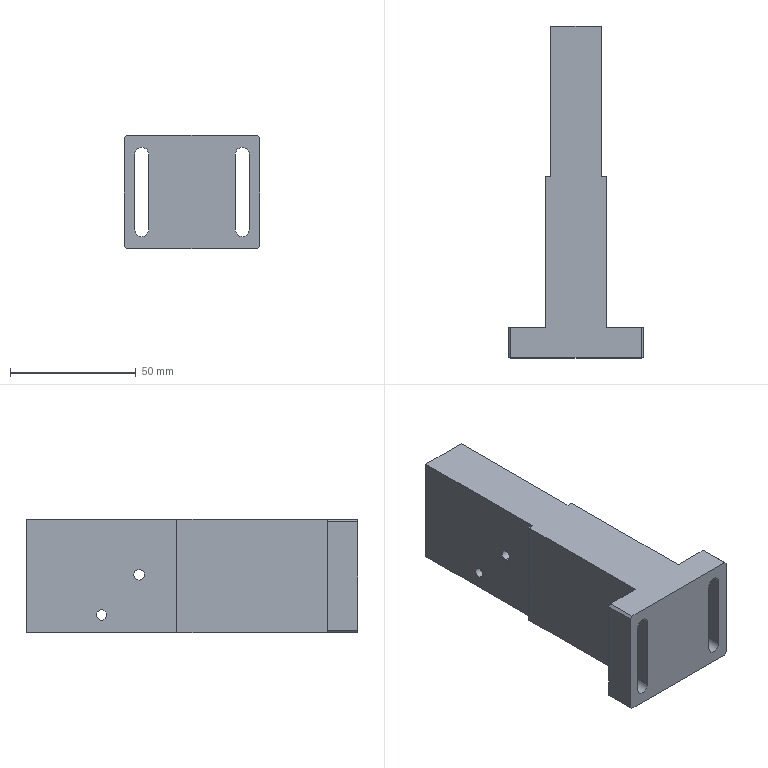Part | SolidWorks | features HoleWzd 3, ICE 2, Chamfer 1, Extrusion 1 | 1 solid | 40 faces | box 54 x 132 x 45 mm | volume 142452 mm3 | plane 22 | cylinder 14 | cone 4 | commonest cylinder face diameters 4.2 x8 5.5 x6
STEP:
#1=CARTESIAN_POINT('',(0.,118.,35.4));
#2=VERTEX_POINT('',#1);
#3=CARTESIAN_POINT('',(0.,118.,39.6));
#4=VERTEX_POINT('',#3);
#5=CARTESIAN_POINT('',(0.,118.,37.5));
#6=DIRECTION('',(0.,1.,0.));
#7=DIRECTION('',(0.,0.,1.));
#8=AXIS2_PLACEMENT_3D('',#5,#6,#7);
#9=CIRCLE('',#8,2.1);
#10=EDGE_CURVE('',#2,#4,#9,.T.);
#11=ORIENTED_EDGE('',*,*,#10,.F.);
#12=CARTESIAN_POINT('',(0.,132.,35.4));
#13=VERTEX_POINT('',#12);
#14=CARTESIAN_POINT('',(0.,132.,35.4));
#15=DIRECTION('',(0.,1.,0.));
#16=VECTOR('',#15,1000.);
#17=LINE('',#14,#16);
#18=EDGE_CURVE('',#2,#13,#17,.T.);
#19=ORIENTED_EDGE('',*,*,#18,.T.);
#20=CARTESIAN_POINT('',(0.,132.,39.6));
#21=VERTEX_POINT('',#20);
#22=CARTESIAN_POINT('',(0.,132.,37.5));
#23=DIRECTION('',(0.,1.,0.));
#24=DIRECTION('',(0.,0.,1.));
#25=AXIS2_PLACEMENT_3D('',#22,#23,#24);
#26=CIRCLE('',#25,2.1);
#27=EDGE_CURVE('',#13,#21,#26,.T.);
#28=ORIENTED_EDGE('',*,*,#27,.T.);
#29=CARTESIAN_POINT('',(0.,132.,39.6));
#30=DIRECTION('',(0.,1.,0.));
#31=VECTOR('',#30,1000.);
#32=LINE('',#29,#31);
#33=EDGE_CURVE('',#4,#21,#32,.T.);
#34=ORIENTED_EDGE('',*,*,#33,.F.);
#35=EDGE_LOOP('',(#11,#19,#28,#34));
#36=FACE_OUTER_BOUND('',#35,.T.);
#37=CARTESIAN_POINT('',(0.,132.,37.5));
#38=DIRECTION('',(0.,1.,0.));
#39=DIRECTION('',(0.,0.,1.));
#40=AXIS2_PLACEMENT_3D('',#37,#38,#39);
#41=CYLINDRICAL_SURFACE('',#40,2.1);
#42=ADVANCED_FACE('',(#36),#41,.F.);
#43=CARTESIAN_POINT('',(0.,116.738,37.5));
#44=VERTEX_POINT('',#43);
#45=CARTESIAN_POINT('',(0.,118.,39.6));
#46=DIRECTION('',(0.,0.515,0.8572));
#47=VECTOR('',#46,1000.);
#48=LINE('',#45,#47);
#49=EDGE_CURVE('',#44,#4,#48,.T.);
#50=ORIENTED_EDGE('',*,*,#49,.F.);
#51=CARTESIAN_POINT('',(0.,118.,35.4));
#52=DIRECTION('',(0.,0.515,-0.8572));
#53=VECTOR('',#52,1000.);
#54=LINE('',#51,#53);
#55=EDGE_CURVE('',#44,#2,#54,.T.);
#56=ORIENTED_EDGE('',*,*,#55,.T.);
#57=ORIENTED_EDGE('',*,*,#10,.T.);
#58=EDGE_LOOP('',(#50,#56,#57));
#59=FACE_OUTER_BOUND('',#58,.T.);
#60=CARTESIAN_POINT('',(0.,118.,37.5));
#61=DIRECTION('',(0.,1.,0.));
#62=DIRECTION('',(0.,0.,1.));
#63=AXIS2_PLACEMENT_3D('',#60,#61,#62);
#64=CONICAL_SURFACE('',#63,2.1,1.03);
#65=ADVANCED_FACE('',(#59),#64,.F.);
#66=CARTESIAN_POINT('',(0.,118.,5.4));
#67=VERTEX_POINT('',#66);
#68=CARTESIAN_POINT('',(0.,118.,9.6));
#69=VERTEX_POINT('',#68);
#70=CARTESIAN_POINT('',(0.,118.,7.5));
#71=DIRECTION('',(0.,1.,0.));
#72=DIRECTION('',(0.,0.,1.));
#73=AXIS2_PLACEMENT_3D('',#70,#71,#72);
#74=CIRCLE('',#73,2.1);
#75=EDGE_CURVE('',#67,#69,#74,.T.);
#76=ORIENTED_EDGE('',*,*,#75,.F.);
#77=CARTESIAN_POINT('',(0.,132.,5.4));
#78=VERTEX_POINT('',#77);
#79=CARTESIAN_POINT('',(0.,132.,5.4));
#80=DIRECTION('',(0.,1.,0.));
#81=VECTOR('',#80,1000.);
#82=LINE('',#79,#81);
#83=EDGE_CURVE('',#67,#78,#82,.T.);
#84=ORIENTED_EDGE('',*,*,#83,.T.);
#85=CARTESIAN_POINT('',(0.,132.,9.6));
#86=VERTEX_POINT('',#85);
#87=CARTESIAN_POINT('',(0.,132.,7.5));
#88=DIRECTION('',(0.,1.,0.));
#89=DIRECTION('',(0.,0.,1.));
#90=AXIS2_PLACEMENT_3D('',#87,#88,#89);
#91=CIRCLE('',#90,2.1);
#92=EDGE_CURVE('',#78,#86,#91,.T.);
#93=ORIENTED_EDGE('',*,*,#92,.T.);
#94=CARTESIAN_POINT('',(0.,132.,9.6));
#95=DIRECTION('',(0.,1.,0.));
#96=VECTOR('',#95,1000.);
#97=LINE('',#94,#96);
#98=EDGE_CURVE('',#69,#86,#97,.T.);
#99=ORIENTED_EDGE('',*,*,#98,.F.);
#100=EDGE_LOOP('',(#76,#84,#93,#99));
#101=FACE_OUTER_BOUND('',#100,.T.);
#102=CARTESIAN_POINT('',(0.,132.,7.5));
#103=DIRECTION('',(0.,1.,0.));
#104=DIRECTION('',(0.,0.,1.));
#105=AXIS2_PLACEMENT_3D('',#102,#103,#104);
#106=CYLINDRICAL_SURFACE('',#105,2.1);
#107=ADVANCED_FACE('',(#101),#106,.F.);
#108=CARTESIAN_POINT('',(0.,116.738,7.5));
#109=VERTEX_POINT('',#108);
#110=CARTESIAN_POINT('',(0.,118.,9.6));
#111=DIRECTION('',(0.,0.515,0.8572));
#112=VECTOR('',#111,1000.);
#113=LINE('',#110,#112);
#114=EDGE_CURVE('',#109,#69,#113,.T.);
#115=ORIENTED_EDGE('',*,*,#114,.F.);
#116=CARTESIAN_POINT('',(0.,118.,5.4));
#117=DIRECTION('',(0.,0.515,-0.8572));
#118=VECTOR('',#117,1000.);
#119=LINE('',#116,#118);
#120=EDGE_CURVE('',#109,#67,#119,.T.);
#121=ORIENTED_EDGE('',*,*,#120,.T.);
#122=ORIENTED_EDGE('',*,*,#75,.T.);
#123=EDGE_LOOP('',(#115,#121,#122));
#124=FACE_OUTER_BOUND('',#123,.T.);
#125=CARTESIAN_POINT('',(0.,118.,7.5));
#126=DIRECTION('',(0.,1.,0.));
#127=DIRECTION('',(0.,0.,1.));
#128=AXIS2_PLACEMENT_3D('',#125,#126,#127);
#129=CONICAL_SURFACE('',#128,2.1,1.03);
#130=ADVANCED_FACE('',(#124),#129,.F.);
#131=CARTESIAN_POINT('',(-20.,0.,40.25));
#132=VERTEX_POINT('',#131);
#133=CARTESIAN_POINT('',(-17.25,0.,37.5));
#134=VERTEX_POINT('',#133);
#135=CARTESIAN_POINT('',(-20.,0.,37.5));
#136=DIRECTION('',(0.,1.,0.));
#137=DIRECTION('',(0.,0.,1.));
#138=AXIS2_PLACEMENT_3D('',#135,#136,#137);
#139=CIRCLE('',#138,2.75);
#140=EDGE_CURVE('',#132,#134,#139,.T.);
#141=ORIENTED_EDGE('',*,*,#140,.F.);
#142=CARTESIAN_POINT('',(-20.,12.,40.25));
#143=VERTEX_POINT('',#142);
#144=CARTESIAN_POINT('',(-20.,12.,40.25));
#145=DIRECTION('',(0.,1.,0.));
#146=VECTOR('',#145,1000.);
#147=LINE('',#144,#146);
#148=EDGE_CURVE('',#132,#143,#147,.T.);
#149=ORIENTED_EDGE('',*,*,#148,.T.);
#150=CARTESIAN_POINT('',(-17.25,12.,37.5));
#151=VERTEX_POINT('',#150);
#152=CARTESIAN_POINT('',(-20.,12.,37.5));
#153=DIRECTION('',(0.,1.,0.));
#154=DIRECTION('',(0.,0.,1.));
#155=AXIS2_PLACEMENT_3D('',#152,#153,#154);
#156=CIRCLE('',#155,2.75);
#157=EDGE_CURVE('',#143,#151,#156,.T.);
#158=ORIENTED_EDGE('',*,*,#157,.T.);
#159=CARTESIAN_POINT('',(-17.25,12.,37.5));
#160=DIRECTION('',(0.,1.,0.));
#161=VECTOR('',#160,1000.);
#162=LINE('',#159,#161);
#163=EDGE_CURVE('',#134,#151,#162,.T.);
#164=ORIENTED_EDGE('',*,*,#163,.F.);
#165=EDGE_LOOP('',(#141,#149,#158,#164));
#166=FACE_OUTER_BOUND('',#165,.T.);
#167=CARTESIAN_POINT('',(-20.,12.,37.5));
#168=DIRECTION('',(0.,1.,0.));
#169=DIRECTION('',(0.,0.,1.));
#170=AXIS2_PLACEMENT_3D('',#167,#168,#169);
#171=CYLINDRICAL_SURFACE('',#170,2.75);
#172=ADVANCED_FACE('',(#166),#171,.F.);
#173=CARTESIAN_POINT('',(20.,0.,40.25));
#174=VERTEX_POINT('',#173);
#175=CARTESIAN_POINT('',(22.75,0.,37.5));
#176=VERTEX_POINT('',#175);
#177=CARTESIAN_POINT('',(20.,0.,37.5));
#178=DIRECTION('',(0.,1.,0.));
#179=DIRECTION('',(0.,0.,1.));
#180=AXIS2_PLACEMENT_3D('',#177,#178,#179);
#181=CIRCLE('',#180,2.75);
#182=EDGE_CURVE('',#174,#176,#181,.T.);
#183=ORIENTED_EDGE('',*,*,#182,.F.);
#184=CARTESIAN_POINT('',(20.,12.,40.25));
#185=VERTEX_POINT('',#184);
#186=CARTESIAN_POINT('',(20.,12.,40.25));
#187=DIRECTION('',(0.,1.,0.));
#188=VECTOR('',#187,1000.);
#189=LINE('',#186,#188);
#190=EDGE_CURVE('',#174,#185,#189,.T.);
#191=ORIENTED_EDGE('',*,*,#190,.T.);
#192=CARTESIAN_POINT('',(22.75,12.,37.5));
#193=VERTEX_POINT('',#192);
#194=CARTESIAN_POINT('',(20.,12.,37.5));
#195=DIRECTION('',(0.,1.,0.));
#196=DIRECTION('',(0.,0.,1.));
#197=AXIS2_PLACEMENT_3D('',#194,#195,#196);
#198=CIRCLE('',#197,2.75);
#199=EDGE_CURVE('',#185,#193,#198,.T.);
#200=ORIENTED_EDGE('',*,*,#199,.T.);
#201=CARTESIAN_POINT('',(22.75,12.,37.5));
#202=DIRECTION('',(0.,1.,0.));
#203=VECTOR('',#202,1000.);
#204=LINE('',#201,#203);
#205=EDGE_CURVE('',#176,#193,#204,.T.);
#206=ORIENTED_EDGE('',*,*,#205,.F.);
#207=EDGE_LOOP('',(#183,#191,#200,#206));
#208=FACE_OUTER_BOUND('',#207,.T.);
#209=CARTESIAN_POINT('',(20.,12.,37.5));
#210=DIRECTION('',(0.,1.,0.));
#211=DIRECTION('',(0.,0.,1.));
#212=AXIS2_PLACEMENT_3D('',#209,#210,#211);
#213=CYLINDRICAL_SURFACE('',#212,2.75);
#214=ADVANCED_FACE('',(#208),#213,.F.);
#215=CARTESIAN_POINT('',(-10.,102.,9.1));
#216=VERTEX_POINT('',#215);
#217=CARTESIAN_POINT('',(-10.,102.,4.9));
#218=VERTEX_POINT('',#217);
#219=CARTESIAN_POINT('',(-10.,102.,7.));
#220=DIRECTION('',(1.,0.,0.));
#221=DIRECTION('',(0.,1.,0.));
#222=AXIS2_PLACEMENT_3D('',#219,#220,#221);
#223=CIRCLE('',#222,2.1);
#224=EDGE_CURVE('',#216,#218,#223,.T.);
#225=ORIENTED_EDGE('',*,*,#224,.F.);
#226=CARTESIAN_POINT('',(10.,102.,9.1));
#227=VERTEX_POINT('',#226);
#228=CARTESIAN_POINT('',(10.,102.,9.1));
#229=DIRECTION('',(1.,0.,0.));
#230=VECTOR('',#229,1000.);
#231=LINE('',#228,#230);
#232=EDGE_CURVE('',#216,#227,#231,.T.);
#233=ORIENTED_EDGE('',*,*,#232,.T.);
#234=CARTESIAN_POINT('',(10.,102.,4.9));
#235=VERTEX_POINT('',#234);
#236=CARTESIAN_POINT('',(10.,102.,7.));
#237=DIRECTION('',(1.,0.,0.));
#238=DIRECTION('',(0.,0.,-1.));
#239=AXIS2_PLACEMENT_3D('',#236,#237,#238);
#240=CIRCLE('',#239,2.1);
#241=EDGE_CURVE('',#227,#235,#240,.T.);
#242=ORIENTED_EDGE('',*,*,#241,.T.);
#243=CARTESIAN_POINT('',(10.,102.,4.9));
#244=DIRECTION('',(1.,0.,0.));
#245=VECTOR('',#244,1000.);
#246=LINE('',#243,#245);
#247=EDGE_CURVE('',#218,#235,#246,.T.);
#248=ORIENTED_EDGE('',*,*,#247,.F.);
#249=EDGE_LOOP('',(#225,#233,#242,#248));
#250=FACE_OUTER_BOUND('',#249,.T.);
#251=CARTESIAN_POINT('',(10.,102.,7.));
#252=DIRECTION('',(1.,0.,0.));
#253=DIRECTION('',(0.,0.,-1.));
#254=AXIS2_PLACEMENT_3D('',#251,#252,#253);
#255=CYLINDRICAL_SURFACE('',#254,2.1);
#256=ADVANCED_FACE('',(#250),#255,.F.);
#257=CARTESIAN_POINT('',(-10.,87.,25.1));
#258=VERTEX_POINT('',#257);
#259=CARTESIAN_POINT('',(-10.,87.,20.9));
#260=VERTEX_POINT('',#259);
#261=CARTESIAN_POINT('',(-10.,87.,23.));
#262=DIRECTION('',(1.,0.,0.));
#263=DIRECTION('',(0.,1.,0.));
#264=AXIS2_PLACEMENT_3D('',#261,#262,#263);
#265=CIRCLE('',#264,2.1);
#266=EDGE_CURVE('',#258,#260,#265,.T.);
#267=ORIENTED_EDGE('',*,*,#266,.F.);
#268=CARTESIAN_POINT('',(10.,87.,25.1));
#269=VERTEX_POINT('',#268);
#270=CARTESIAN_POINT('',(10.,87.,25.1));
#271=DIRECTION('',(1.,0.,0.));
#272=VECTOR('',#271,1000.);
#273=LINE('',#270,#272);
#274=EDGE_CURVE('',#258,#269,#273,.T.);
#275=ORIENTED_EDGE('',*,*,#274,.T.);
#276=CARTESIAN_POINT('',(10.,87.,20.9));
#277=VERTEX_POINT('',#276);
#278=CARTESIAN_POINT('',(10.,87.,23.));
#279=DIRECTION('',(1.,0.,0.));
#280=DIRECTION('',(0.,0.,-1.));
#281=AXIS2_PLACEMENT_3D('',#278,#279,#280);
#282=CIRCLE('',#281,2.1);
#283=EDGE_CURVE('',#269,#277,#282,.T.);
#284=ORIENTED_EDGE('',*,*,#283,.T.);
#285=CARTESIAN_POINT('',(10.,87.,20.9));
#286=DIRECTION('',(1.,0.,0.));
#287=VECTOR('',#286,1000.);
#288=LINE('',#285,#287);
#289=EDGE_CURVE('',#260,#277,#288,.T.);
#290=ORIENTED_EDGE('',*,*,#289,.F.);
#291=EDGE_LOOP('',(#267,#275,#284,#290));
#292=FACE_OUTER_BOUND('',#291,.T.);
#293=CARTESIAN_POINT('',(10.,87.,23.));
#294=DIRECTION('',(1.,0.,0.));
#295=DIRECTION('',(0.,0.,-1.));
#296=AXIS2_PLACEMENT_3D('',#293,#294,#295);
#297=CYLINDRICAL_SURFACE('',#296,2.1);
#298=ADVANCED_FACE('',(#292),#297,.F.);
#299=CARTESIAN_POINT('',(22.75,0.,7.5));
#300=VERTEX_POINT('',#299);
#301=CARTESIAN_POINT('',(22.75,12.,7.5));
#302=VERTEX_POINT('',#301);
#303=CARTESIAN_POINT('',(22.75,12.,7.5));
#304=DIRECTION('',(0.,1.,0.));
#305=VECTOR('',#304,1000.);
#306=LINE('',#303,#305);
#307=EDGE_CURVE('',#300,#302,#306,.T.);
#308=ORIENTED_EDGE('',*,*,#307,.T.);
#309=CARTESIAN_POINT('',(17.25,12.,7.5));
#310=VERTEX_POINT('',#309);
#311=CARTESIAN_POINT('',(20.,12.,7.5));
#312=DIRECTION('',(0.,1.,0.));
#313=DIRECTION('',(0.,0.,1.));
#314=AXIS2_PLACEMENT_3D('',#311,#312,#313);
#315=CIRCLE('',#314,2.75);
#316=EDGE_CURVE('',#302,#310,#315,.T.);
#317=ORIENTED_EDGE('',*,*,#316,.T.);
#318=CARTESIAN_POINT('',(17.25,0.,7.5));
#319=VERTEX_POINT('',#318);
#320=CARTESIAN_POINT('',(17.25,12.,7.5));
#321=DIRECTION('',(0.,1.,0.));
#322=VECTOR('',#321,1000.);
#323=LINE('',#320,#322);
#324=EDGE_CURVE('',#319,#310,#323,.T.);
#325=ORIENTED_EDGE('',*,*,#324,.F.);
#326=CARTESIAN_POINT('',(20.,0.,7.5));
#327=DIRECTION('',(0.,1.,0.));
#328=DIRECTION('',(0.,0.,1.));
#329=AXIS2_PLACEMENT_3D('',#326,#327,#328);
#330=CIRCLE('',#329,2.75);
#331=EDGE_CURVE('',#300,#319,#330,.T.);
#332=ORIENTED_EDGE('',*,*,#331,.F.);
#333=EDGE_LOOP('',(#308,#317,#325,#332));
#334=FACE_OUTER_BOUND('',#333,.T.);
#335=CARTESIAN_POINT('',(20.,12.,7.5));
#336=DIRECTION('',(0.,1.,0.));
#337=DIRECTION('',(0.,0.,1.));
#338=AXIS2_PLACEMENT_3D('',#335,#336,#337);
#339=CYLINDRICAL_SURFACE('',#338,2.75);
#340=ADVANCED_FACE('',(#334),#339,.F.);
#341=CARTESIAN_POINT('',(-17.25,0.,7.5));
#342=VERTEX_POINT('',#341);
#343=CARTESIAN_POINT('',(-17.25,12.,7.5));
#344=VERTEX_POINT('',#343);
#345=CARTESIAN_POINT('',(-17.25,12.,7.5));
#346=DIRECTION('',(0.,1.,0.));
#347=VECTOR('',#346,1000.);
#348=LINE('',#345,#347);
#349=EDGE_CURVE('',#342,#344,#348,.T.);
#350=ORIENTED_EDGE('',*,*,#349,.T.);
#351=CARTESIAN_POINT('',(-22.75,12.,7.5));
#352=VERTEX_POINT('',#351);
#353=CARTESIAN_POINT('',(-20.,12.,7.5));
#354=DIRECTION('',(0.,1.,0.));
#355=DIRECTION('',(0.,0.,1.));
#356=AXIS2_PLACEMENT_3D('',#353,#354,#355);
#357=CIRCLE('',#356,2.75);
#358=EDGE_CURVE('',#344,#352,#357,.T.);
#359=ORIENTED_EDGE('',*,*,#358,.T.);
#360=CARTESIAN_POINT('',(-22.75,0.,7.5));
#361=VERTEX_POINT('',#360);
#362=CARTESIAN_POINT('',(-22.75,12.,7.5));
#363=DIRECTION('',(0.,1.,0.));
#364=VECTOR('',#363,1000.);
#365=LINE('',#362,#364);
#366=EDGE_CURVE('',#361,#352,#365,.T.);
#367=ORIENTED_EDGE('',*,*,#366,.F.);
#368=CARTESIAN_POINT('',(-20.,0.,7.5));
#369=DIRECTION('',(0.,1.,0.));
#370=DIRECTION('',(0.,0.,1.));
#371=AXIS2_PLACEMENT_3D('',#368,#369,#370);
#372=CIRCLE('',#371,2.75);
#373=EDGE_CURVE('',#342,#361,#372,.T.);
#374=ORIENTED_EDGE('',*,*,#373,.F.);
#375=EDGE_LOOP('',(#350,#359,#367,#374));
#376=FACE_OUTER_BOUND('',#375,.T.);
#377=CARTESIAN_POINT('',(-20.,12.,7.5));
#378=DIRECTION('',(0.,1.,0.));
#379=DIRECTION('',(0.,0.,1.));
#380=AXIS2_PLACEMENT_3D('',#377,#378,#379);
#381=CYLINDRICAL_SURFACE('',#380,2.75);
#382=ADVANCED_FACE('',(#376),#381,.F.);
#383=CARTESIAN_POINT('',(-27.,0.,44.));
#384=VERTEX_POINT('',#383);
#385=CARTESIAN_POINT('',(-27.,0.,1.));
#386=VERTEX_POINT('',#385);
#387=CARTESIAN_POINT('',(-27.,0.,45.));
#388=DIRECTION('',(0.,0.,-1.));
#389=VECTOR('',#388,1000.);
#390=LINE('',#387,#389);
#391=EDGE_CURVE('',#384,#386,#390,.T.);
#392=ORIENTED_EDGE('',*,*,#391,.F.);
#393=CARTESIAN_POINT('',(-27.,12.,44.));
#394=VERTEX_POINT('',#393);
#395=CARTESIAN_POINT('',(-27.,0.,44.));
#396=DIRECTION('',(0.,1.,0.));
#397=VECTOR('',#396,1000.);
#398=LINE('',#395,#397);
#399=EDGE_CURVE('',#384,#394,#398,.T.);
#400=ORIENTED_EDGE('',*,*,#399,.T.);
#401=CARTESIAN_POINT('',(-27.,12.,1.));
#402=VERTEX_POINT('',#401);
#403=CARTESIAN_POINT('',(-27.,12.,45.));
#404=DIRECTION('',(0.,0.,-1.));
#405=VECTOR('',#404,1000.);
#406=LINE('',#403,#405);
#407=EDGE_CURVE('',#394,#402,#406,.T.);
#408=ORIENTED_EDGE('',*,*,#407,.T.);
#409=CARTESIAN_POINT('',(-27.,0.,1.));
#410=DIRECTION('',(0.,-1.,0.));
#411=VECTOR('',#410,1000.);
#412=LINE('',#409,#411);
#413=EDGE_CURVE('',#402,#386,#412,.T.);
#414=ORIENTED_EDGE('',*,*,#413,.T.);
#415=EDGE_LOOP('',(#392,#400,#408,#414));
#416=FACE_OUTER_BOUND('',#415,.T.);
#417=CARTESIAN_POINT('',(-27.,0.,45.));
#418=DIRECTION('',(1.,0.,0.));
#419=DIRECTION('',(0.,0.,-1.));
#420=AXIS2_PLACEMENT_3D('',#417,#418,#419);
#421=PLANE('',#420);
#422=ADVANCED_FACE('',(#416),#421,.F.);
#423=CARTESIAN_POINT('',(-22.75,0.,37.5));
#424=VERTEX_POINT('',#423);
#425=CARTESIAN_POINT('',(-20.,0.,37.5));
#426=DIRECTION('',(0.,1.,0.));
#427=DIRECTION('',(0.,0.,1.));
#428=AXIS2_PLACEMENT_3D('',#425,#426,#427);
#429=CIRCLE('',#428,2.75);
#430=EDGE_CURVE('',#424,#132,#429,.T.);
#431=ORIENTED_EDGE('',*,*,#430,.T.);
#432=ORIENTED_EDGE('',*,*,#140,.T.);
#433=CARTESIAN_POINT('',(-17.25,0.,37.5));
#434=DIRECTION('',(0.,0.,1.));
#435=VECTOR('',#434,1000.);
#436=LINE('',#433,#435);
#437=EDGE_CURVE('',#342,#134,#436,.T.);
#438=ORIENTED_EDGE('',*,*,#437,.F.);
#439=ORIENTED_EDGE('',*,*,#373,.T.);
#440=CARTESIAN_POINT('',(-22.75,0.,37.5));
#441=DIRECTION('',(0.,0.,-1.));
#442=VECTOR('',#441,1000.);
#443=LINE('',#440,#442);
#444=EDGE_CURVE('',#424,#361,#443,.T.);
#445=ORIENTED_EDGE('',*,*,#444,.F.);
#446=EDGE_LOOP('',(#431,#432,#438,#439,#445));
#447=FACE_BOUND('',#446,.T.);
#448=CARTESIAN_POINT('',(17.25,0.,37.5));
#449=VERTEX_POINT('',#448);
#450=CARTESIAN_POINT('',(20.,0.,37.5));
#451=DIRECTION('',(0.,1.,0.));
#452=DIRECTION('',(0.,0.,1.));
#453=AXIS2_PLACEMENT_3D('',#450,#451,#452);
#454=CIRCLE('',#453,2.75);
#455=EDGE_CURVE('',#449,#174,#454,.T.);
#456=ORIENTED_EDGE('',*,*,#455,.T.);
#457=ORIENTED_EDGE('',*,*,#182,.T.);
#458=CARTESIAN_POINT('',(22.75,0.,37.5));
#459=DIRECTION('',(0.,0.,1.));
#460=VECTOR('',#459,1000.);
#461=LINE('',#458,#460);
#462=EDGE_CURVE('',#300,#176,#461,.T.);
#463=ORIENTED_EDGE('',*,*,#462,.F.);
#464=ORIENTED_EDGE('',*,*,#331,.T.);
#465=CARTESIAN_POINT('',(17.25,0.,37.5));
#466=DIRECTION('',(0.,0.,-1.));
#467=VECTOR('',#466,1000.);
#468=LINE('',#465,#467);
#469=EDGE_CURVE('',#449,#319,#468,.T.);
#470=ORIENTED_EDGE('',*,*,#469,.F.);
#471=EDGE_LOOP('',(#456,#457,#463,#464,#470));
#472=FACE_BOUND('',#471,.T.);
#473=CARTESIAN_POINT('',(-26.,0.,45.));
#474=VERTEX_POINT('',#473);
#475=CARTESIAN_POINT('',(26.,0.,45.));
#476=VERTEX_POINT('',#475);
#477=CARTESIAN_POINT('',(27.,0.,45.));
#478=DIRECTION('',(1.,0.,0.));
#479=VECTOR('',#478,1000.);
#480=LINE('',#477,#479);
#481=EDGE_CURVE('',#474,#476,#480,.T.);
#482=ORIENTED_EDGE('',*,*,#481,.F.);
#483=CARTESIAN_POINT('',(-26.,0.,45.));
#484=DIRECTION('',(-0.7071,0.,-0.7071));
#485=VECTOR('',#484,1000.);
#486=LINE('',#483,#485);
#487=EDGE_CURVE('',#474,#384,#486,.T.);
#488=ORIENTED_EDGE('',*,*,#487,.T.);
#489=ORIENTED_EDGE('',*,*,#391,.T.);
#490=CARTESIAN_POINT('',(-26.,0.,0.));
#491=VERTEX_POINT('',#490);
#492=CARTESIAN_POINT('',(-27.,0.,1.));
#493=DIRECTION('',(0.7071,0.,-0.7071));
#494=VECTOR('',#493,1000.);
#495=LINE('',#492,#494);
#496=EDGE_CURVE('',#386,#491,#495,.T.);
#497=ORIENTED_EDGE('',*,*,#496,.T.);
#498=CARTESIAN_POINT('',(26.,0.,0.));
#499=VERTEX_POINT('',#498);
#500=CARTESIAN_POINT('',(27.,0.,0.));
#501=DIRECTION('',(1.,0.,0.));
#502=VECTOR('',#501,1000.);
#503=LINE('',#500,#502);
#504=EDGE_CURVE('',#491,#499,#503,.T.);
#505=ORIENTED_EDGE('',*,*,#504,.T.);
#506=CARTESIAN_POINT('',(27.,0.,1.));
#507=VERTEX_POINT('',#506);
#508=CARTESIAN_POINT('',(27.,0.,1.));
#509=DIRECTION('',(0.7071,0.,0.7071));
#510=VECTOR('',#509,1000.);
#511=LINE('',#508,#510);
#512=EDGE_CURVE('',#499,#507,#511,.T.);
#513=ORIENTED_EDGE('',*,*,#512,.T.);
#514=CARTESIAN_POINT('',(27.,0.,44.));
#515=VERTEX_POINT('',#514);
#516=CARTESIAN_POINT('',(27.,0.,45.));
#517=DIRECTION('',(0.,0.,-1.));
#518=VECTOR('',#517,1000.);
#519=LINE('',#516,#518);
#520=EDGE_CURVE('',#515,#507,#519,.T.);
#521=ORIENTED_EDGE('',*,*,#520,.F.);
#522=CARTESIAN_POINT('',(26.,0.,45.));
#523=DIRECTION('',(-0.7071,0.,0.7071));
#524=VECTOR('',#523,1000.);
#525=LINE('',#522,#524);
#526=EDGE_CURVE('',#515,#476,#525,.T.);
#527=ORIENTED_EDGE('',*,*,#526,.T.);
#528=EDGE_LOOP('',(#482,#488,#489,#497,#505,#513,#521,#527));
#529=FACE_OUTER_BOUND('',#528,.T.);
#530=CARTESIAN_POINT('',(27.,0.,45.));
#531=DIRECTION('',(0.,1.,0.));
#532=DIRECTION('',(0.,0.,1.));
#533=AXIS2_PLACEMENT_3D('',#530,#531,#532);
#534=PLANE('',#533);
#535=ADVANCED_FACE('',(#447,#472,#529),#534,.F.);
#536=CARTESIAN_POINT('',(27.,12.,44.));
#537=VERTEX_POINT('',#536);
#538=CARTESIAN_POINT('',(27.,12.,1.));
#539=VERTEX_POINT('',#538);
#540=CARTESIAN_POINT('',(27.,12.,45.));
#541=DIRECTION('',(0.,0.,-1.));
#542=VECTOR('',#541,1000.);
#543=LINE('',#540,#542);
#544=EDGE_CURVE('',#537,#539,#543,.T.);
#545=ORIENTED_EDGE('',*,*,#544,.F.);
#546=CARTESIAN_POINT('',(27.,0.,44.));
#547=DIRECTION('',(0.,-1.,0.));
#548=VECTOR('',#547,1000.);
#549=LINE('',#546,#548);
#550=EDGE_CURVE('',#537,#515,#549,.T.);
#551=ORIENTED_EDGE('',*,*,#550,.T.);
#552=ORIENTED_EDGE('',*,*,#520,.T.);
#553=CARTESIAN_POINT('',(27.,12.,1.));
#554=DIRECTION('',(0.,1.,0.));
#555=VECTOR('',#554,1000.);
#556=LINE('',#553,#555);
#557=EDGE_CURVE('',#507,#539,#556,.T.);
#558=ORIENTED_EDGE('',*,*,#557,.T.);
#559=EDGE_LOOP('',(#545,#551,#552,#558));
#560=FACE_OUTER_BOUND('',#559,.T.);
#561=CARTESIAN_POINT('',(27.,0.,45.));
#562=DIRECTION('',(-1.,0.,0.));
#563=DIRECTION('',(0.,0.,1.));
#564=AXIS2_PLACEMENT_3D('',#561,#562,#563);
#565=PLANE('',#564);
#566=ADVANCED_FACE('',(#560),#565,.F.);
#567=ORIENTED_EDGE('',*,*,#316,.F.);
#568=CARTESIAN_POINT('',(22.75,12.,37.5));
#569=DIRECTION('',(0.,0.,-1.));
#570=VECTOR('',#569,1000.);
#571=LINE('',#568,#570);
#572=EDGE_CURVE('',#193,#302,#571,.T.);
#573=ORIENTED_EDGE('',*,*,#572,.F.);
#574=ORIENTED_EDGE('',*,*,#199,.F.);
#575=CARTESIAN_POINT('',(17.25,12.,37.5));
#576=VERTEX_POINT('',#575);
#577=CARTESIAN_POINT('',(20.,12.,37.5));
#578=DIRECTION('',(0.,1.,0.));
#579=DIRECTION('',(0.,0.,1.));
#580=AXIS2_PLACEMENT_3D('',#577,#578,#579);
#581=CIRCLE('',#580,2.75);
#582=EDGE_CURVE('',#576,#185,#581,.T.);
#583=ORIENTED_EDGE('',*,*,#582,.F.);
#584=CARTESIAN_POINT('',(17.25,12.,37.5));
#585=DIRECTION('',(0.,0.,1.));
#586=VECTOR('',#585,1000.);
#587=LINE('',#584,#586);
#588=EDGE_CURVE('',#310,#576,#587,.T.);
#589=ORIENTED_EDGE('',*,*,#588,.F.);
#590=EDGE_LOOP('',(#567,#573,#574,#583,#589));
#591=FACE_BOUND('',#590,.T.);
#592=CARTESIAN_POINT('',(26.,12.,45.));
#593=VERTEX_POINT('',#592);
#594=CARTESIAN_POINT('',(12.,12.,45.));
#595=VERTEX_POINT('',#594);
#596=CARTESIAN_POINT('',(27.,12.,45.));
#597=DIRECTION('',(-1.,0.,0.));
#598=VECTOR('',#597,1000.);
#599=LINE('',#596,#598);
#600=EDGE_CURVE('',#593,#595,#599,.T.);
#601=ORIENTED_EDGE('',*,*,#600,.F.);
#602=CARTESIAN_POINT('',(26.,12.,45.));
#603=DIRECTION('',(0.7071,0.,-0.7071));
#604=VECTOR('',#603,1000.);
#605=LINE('',#602,#604);
#606=EDGE_CURVE('',#593,#537,#605,.T.);
#607=ORIENTED_EDGE('',*,*,#606,.T.);
#608=ORIENTED_EDGE('',*,*,#544,.T.);
#609=CARTESIAN_POINT('',(26.,12.,0.));
#610=VERTEX_POINT('',#609);
#611=CARTESIAN_POINT('',(27.,12.,1.));
#612=DIRECTION('',(-0.7071,0.,-0.7071));
#613=VECTOR('',#612,1000.);
#614=LINE('',#611,#613);
#615=EDGE_CURVE('',#539,#610,#614,.T.);
#616=ORIENTED_EDGE('',*,*,#615,.T.);
#617=CARTESIAN_POINT('',(12.,12.,0.));
#618=VERTEX_POINT('',#617);
#619=CARTESIAN_POINT('',(27.,12.,0.));
#620=DIRECTION('',(-1.,0.,0.));
#621=VECTOR('',#620,1000.);
#622=LINE('',#619,#621);
#623=EDGE_CURVE('',#610,#618,#622,.T.);
#624=ORIENTED_EDGE('',*,*,#623,.T.);
#625=CARTESIAN_POINT('',(12.,12.,45.));
#626=DIRECTION('',(0.,0.,-1.));
#627=VECTOR('',#626,1000.);
#628=LINE('',#625,#627);
#629=EDGE_CURVE('',#595,#618,#628,.T.);
#630=ORIENTED_EDGE('',*,*,#629,.F.);
#631=EDGE_LOOP('',(#601,#607,#608,#616,#624,#630));
#632=FACE_OUTER_BOUND('',#631,.T.);
#633=CARTESIAN_POINT('',(27.,12.,45.));
#634=DIRECTION('',(0.,-1.,0.));
#635=DIRECTION('',(0.,0.,-1.));
#636=AXIS2_PLACEMENT_3D('',#633,#634,#635);
#637=PLANE('',#636);
#638=ADVANCED_FACE('',(#591,#632),#637,.F.);
#639=CARTESIAN_POINT('',(12.,72.,0.));
#640=VERTEX_POINT('',#639);
#641=CARTESIAN_POINT('',(12.,12.,0.));
#642=DIRECTION('',(0.,1.,0.));
#643=VECTOR('',#642,1000.);
#644=LINE('',#641,#643);
#645=EDGE_CURVE('',#618,#640,#644,.T.);
#646=ORIENTED_EDGE('',*,*,#645,.T.);
#647=CARTESIAN_POINT('',(12.,72.,45.));
#648=VERTEX_POINT('',#647);
#649=CARTESIAN_POINT('',(12.,72.,0.));
#650=DIRECTION('',(0.,0.,1.));
#651=VECTOR('',#650,1000.);
#652=LINE('',#649,#651);
#653=EDGE_CURVE('',#640,#648,#652,.T.);
#654=ORIENTED_EDGE('',*,*,#653,.T.);
#655=CARTESIAN_POINT('',(12.,12.,45.));
#656=DIRECTION('',(0.,1.,0.));
#657=VECTOR('',#656,1000.);
#658=LINE('',#655,#657);
#659=EDGE_CURVE('',#595,#648,#658,.T.);
#660=ORIENTED_EDGE('',*,*,#659,.F.);
#661=ORIENTED_EDGE('',*,*,#629,.T.);
#662=EDGE_LOOP('',(#646,#654,#660,#661));
#663=FACE_OUTER_BOUND('',#662,.T.);
#664=CARTESIAN_POINT('',(12.,12.,45.));
#665=DIRECTION('',(-1.,0.,0.));
#666=DIRECTION('',(0.,0.,1.));
#667=AXIS2_PLACEMENT_3D('',#664,#665,#666);
#668=PLANE('',#667);
#669=ADVANCED_FACE('',(#663),#668,.F.);
#670=CARTESIAN_POINT('',(0.,132.,37.5));
#671=DIRECTION('',(0.,1.,0.));
#672=DIRECTION('',(0.,0.,1.));
#673=AXIS2_PLACEMENT_3D('',#670,#671,#672);
#674=CIRCLE('',#673,2.1);
#675=EDGE_CURVE('',#21,#13,#674,.T.);
#676=ORIENTED_EDGE('',*,*,#675,.F.);
#677=ORIENTED_EDGE('',*,*,#27,.F.);
#678=EDGE_LOOP('',(#676,#677));
#679=FACE_BOUND('',#678,.T.);
#680=CARTESIAN_POINT('',(0.,132.,7.5));
#681=DIRECTION('',(0.,1.,0.));
#682=DIRECTION('',(0.,0.,1.));
#683=AXIS2_PLACEMENT_3D('',#680,#681,#682);
#684=CIRCLE('',#683,2.1);
#685=EDGE_CURVE('',#86,#78,#684,.T.);
#686=ORIENTED_EDGE('',*,*,#685,.F.);
#687=ORIENTED_EDGE('',*,*,#92,.F.);
#688=EDGE_LOOP('',(#686,#687));
#689=FACE_BOUND('',#688,.T.);
#690=CARTESIAN_POINT('',(10.,132.,45.));
#691=VERTEX_POINT('',#690);
#692=CARTESIAN_POINT('',(-10.,132.,45.));
#693=VERTEX_POINT('',#692);
#694=CARTESIAN_POINT('',(-12.,132.,45.));
#695=DIRECTION('',(-1.,0.,0.));
#696=VECTOR('',#695,1000.);
#697=LINE('',#694,#696);
#698=EDGE_CURVE('',#691,#693,#697,.T.);
#699=ORIENTED_EDGE('',*,*,#698,.F.);
#700=CARTESIAN_POINT('',(10.,132.,0.));
#701=VERTEX_POINT('',#700);
#702=CARTESIAN_POINT('',(10.,132.,0.));
#703=DIRECTION('',(0.,0.,1.));
#704=VECTOR('',#703,1000.);
#705=LINE('',#702,#704);
#706=EDGE_CURVE('',#701,#691,#705,.T.);
#707=ORIENTED_EDGE('',*,*,#706,.F.);
#708=CARTESIAN_POINT('',(-10.,132.,0.));
#709=VERTEX_POINT('',#708);
#710=CARTESIAN_POINT('',(-12.,132.,0.));
#711=DIRECTION('',(-1.,0.,0.));
#712=VECTOR('',#711,1000.);
#713=LINE('',#710,#712);
#714=EDGE_CURVE('',#701,#709,#713,.T.);
#715=ORIENTED_EDGE('',*,*,#714,.T.);
#716=CARTESIAN_POINT('',(-10.,132.,0.));
#717=DIRECTION('',(0.,0.,1.));
#718=VECTOR('',#717,1000.);
#719=LINE('',#716,#718);
#720=EDGE_CURVE('',#709,#693,#719,.T.);
#721=ORIENTED_EDGE('',*,*,#720,.T.);
#722=EDGE_LOOP('',(#699,#707,#715,#721));
#723=FACE_OUTER_BOUND('',#722,.T.);
#724=CARTESIAN_POINT('',(-12.,132.,45.));
#725=DIRECTION('',(0.,-1.,0.));
#726=DIRECTION('',(0.,0.,-1.));
#727=AXIS2_PLACEMENT_3D('',#724,#725,#726);
#728=PLANE('',#727);
#729=ADVANCED_FACE('',(#679,#689,#723),#728,.F.);
#730=CARTESIAN_POINT('',(-12.,72.,45.));
#731=VERTEX_POINT('',#730);
#732=CARTESIAN_POINT('',(-12.,12.,45.));
#733=VERTEX_POINT('',#732);
#734=CARTESIAN_POINT('',(-12.,12.,45.));
#735=DIRECTION('',(0.,-1.,0.));
#736=VECTOR('',#735,1000.);
#737=LINE('',#734,#736);
#738=EDGE_CURVE('',#731,#733,#737,.T.);
#739=ORIENTED_EDGE('',*,*,#738,.F.);
#740=CARTESIAN_POINT('',(-12.,72.,0.));
#741=VERTEX_POINT('',#740);
#742=CARTESIAN_POINT('',(-12.,72.,0.));
#743=DIRECTION('',(0.,0.,1.));
#744=VECTOR('',#743,1000.);
#745=LINE('',#742,#744);
#746=EDGE_CURVE('',#741,#731,#745,.T.);
#747=ORIENTED_EDGE('',*,*,#746,.F.);
#748=CARTESIAN_POINT('',(-12.,12.,0.));
#749=VERTEX_POINT('',#748);
#750=CARTESIAN_POINT('',(-12.,12.,0.));
#751=DIRECTION('',(0.,-1.,0.));
#752=VECTOR('',#751,1000.);
#753=LINE('',#750,#752);
#754=EDGE_CURVE('',#741,#749,#753,.T.);
#755=ORIENTED_EDGE('',*,*,#754,.T.);
#756=CARTESIAN_POINT('',(-12.,12.,45.));
#757=DIRECTION('',(0.,0.,-1.));
#758=VECTOR('',#757,1000.);
#759=LINE('',#756,#758);
#760=EDGE_CURVE('',#733,#749,#759,.T.);
#761=ORIENTED_EDGE('',*,*,#760,.F.);
#762=EDGE_LOOP('',(#739,#747,#755,#761));
#763=FACE_OUTER_BOUND('',#762,.T.);
#764=CARTESIAN_POINT('',(-12.,12.,45.));
#765=DIRECTION('',(1.,0.,0.));
#766=DIRECTION('',(0.,0.,-1.));
#767=AXIS2_PLACEMENT_3D('',#764,#765,#766);
#768=PLANE('',#767);
#769=ADVANCED_FACE('',(#763),#768,.F.);
#770=ORIENTED_EDGE('',*,*,#358,.F.);
#771=CARTESIAN_POINT('',(-17.25,12.,37.5));
#772=DIRECTION('',(0.,0.,-1.));
#773=VECTOR('',#772,1000.);
#774=LINE('',#771,#773);
#775=EDGE_CURVE('',#151,#344,#774,.T.);
#776=ORIENTED_EDGE('',*,*,#775,.F.);
#777=ORIENTED_EDGE('',*,*,#157,.F.);
#778=CARTESIAN_POINT('',(-22.75,12.,37.5));
#779=VERTEX_POINT('',#778);
#780=CARTESIAN_POINT('',(-20.,12.,37.5));
#781=DIRECTION('',(0.,1.,0.));
#782=DIRECTION('',(0.,0.,1.));
#783=AXIS2_PLACEMENT_3D('',#780,#781,#782);
#784=CIRCLE('',#783,2.75);
#785=EDGE_CURVE('',#779,#143,#784,.T.);
#786=ORIENTED_EDGE('',*,*,#785,.F.);
#787=CARTESIAN_POINT('',(-22.75,12.,37.5));
#788=DIRECTION('',(0.,0.,1.));
#789=VECTOR('',#788,1000.);
#790=LINE('',#787,#789);
#791=EDGE_CURVE('',#352,#779,#790,.T.);
#792=ORIENTED_EDGE('',*,*,#791,.F.);
#793=EDGE_LOOP('',(#770,#776,#777,#786,#792));
#794=FACE_BOUND('',#793,.T.);
#795=ORIENTED_EDGE('',*,*,#407,.F.);
#796=CARTESIAN_POINT('',(-26.,12.,45.));
#797=VERTEX_POINT('',#796);
#798=CARTESIAN_POINT('',(-26.,12.,45.));
#799=DIRECTION('',(0.7071,0.,0.7071));
#800=VECTOR('',#799,1000.);
#801=LINE('',#798,#800);
#802=EDGE_CURVE('',#394,#797,#801,.T.);
#803=ORIENTED_EDGE('',*,*,#802,.T.);
#804=CARTESIAN_POINT('',(-27.,12.,45.));
#805=DIRECTION('',(-1.,0.,0.));
#806=VECTOR('',#805,1000.);
#807=LINE('',#804,#806);
#808=EDGE_CURVE('',#733,#797,#807,.T.);
#809=ORIENTED_EDGE('',*,*,#808,.F.);
#810=ORIENTED_EDGE('',*,*,#760,.T.);
#811=CARTESIAN_POINT('',(-26.,12.,0.));
#812=VERTEX_POINT('',#811);
#813=CARTESIAN_POINT('',(-27.,12.,0.));
#814=DIRECTION('',(-1.,0.,0.));
#815=VECTOR('',#814,1000.);
#816=LINE('',#813,#815);
#817=EDGE_CURVE('',#749,#812,#816,.T.);
#818=ORIENTED_EDGE('',*,*,#817,.T.);
#819=CARTESIAN_POINT('',(-27.,12.,1.));
#820=DIRECTION('',(-0.7071,0.,0.7071));
#821=VECTOR('',#820,1000.);
#822=LINE('',#819,#821);
#823=EDGE_CURVE('',#812,#402,#822,.T.);
#824=ORIENTED_EDGE('',*,*,#823,.T.);
#825=EDGE_LOOP('',(#795,#803,#809,#810,#818,#824));
#826=FACE_OUTER_BOUND('',#825,.T.);
#827=CARTESIAN_POINT('',(-27.,12.,45.));
#828=DIRECTION('',(0.,-1.,0.));
#829=DIRECTION('',(0.,0.,-1.));
#830=AXIS2_PLACEMENT_3D('',#827,#828,#829);
#831=PLANE('',#830);
#832=ADVANCED_FACE('',(#794,#826),#831,.F.);
#833=ORIENTED_EDGE('',*,*,#808,.T.);
#834=CARTESIAN_POINT('',(-26.,12.,45.));
#835=DIRECTION('',(0.,-1.,0.));
#836=VECTOR('',#835,1000.);
#837=LINE('',#834,#836);
#838=EDGE_CURVE('',#797,#474,#837,.T.);
#839=ORIENTED_EDGE('',*,*,#838,.T.);
#840=ORIENTED_EDGE('',*,*,#481,.T.);
#841=CARTESIAN_POINT('',(26.,12.,45.));
#842=DIRECTION('',(0.,1.,0.));
#843=VECTOR('',#842,1000.);
#844=LINE('',#841,#843);
#845=EDGE_CURVE('',#476,#593,#844,.T.);
#846=ORIENTED_EDGE('',*,*,#845,.T.);
#847=ORIENTED_EDGE('',*,*,#600,.T.);
#848=ORIENTED_EDGE('',*,*,#659,.T.);
#849=CARTESIAN_POINT('',(10.,72.,45.));
#850=VERTEX_POINT('',#849);
#851=CARTESIAN_POINT('',(12.,72.,45.));
#852=DIRECTION('',(1.,0.,0.));
#853=VECTOR('',#852,1000.);
#854=LINE('',#851,#853);
#855=EDGE_CURVE('',#850,#648,#854,.T.);
#856=ORIENTED_EDGE('',*,*,#855,.F.);
#857=CARTESIAN_POINT('',(10.,132.,45.));
#858=DIRECTION('',(0.,-1.,0.));
#859=VECTOR('',#858,1000.);
#860=LINE('',#857,#859);
#861=EDGE_CURVE('',#691,#850,#860,.T.);
#862=ORIENTED_EDGE('',*,*,#861,.F.);
#863=ORIENTED_EDGE('',*,*,#698,.T.);
#864=CARTESIAN_POINT('',(-10.,72.,45.));
#865=VERTEX_POINT('',#864);
#866=CARTESIAN_POINT('',(-10.,132.,45.));
#867=DIRECTION('',(0.,1.,0.));
#868=VECTOR('',#867,1000.);
#869=LINE('',#866,#868);
#870=EDGE_CURVE('',#865,#693,#869,.T.);
#871=ORIENTED_EDGE('',*,*,#870,.F.);
#872=CARTESIAN_POINT('',(-12.,72.,45.));
#873=DIRECTION('',(1.,0.,0.));
#874=VECTOR('',#873,1000.);
#875=LINE('',#872,#874);
#876=EDGE_CURVE('',#731,#865,#875,.T.);
#877=ORIENTED_EDGE('',*,*,#876,.F.);
#878=ORIENTED_EDGE('',*,*,#738,.T.);
#879=EDGE_LOOP('',(#833,#839,#840,#846,#847,#848,#856,#862,#863,#871,#877,#878));
#880=FACE_OUTER_BOUND('',#879,.T.);
#881=CARTESIAN_POINT('',(-27.,12.,45.));
#882=DIRECTION('',(0.,0.,-1.));
#883=DIRECTION('',(-1.,0.,0.));
#884=AXIS2_PLACEMENT_3D('',#881,#882,#883);
#885=PLANE('',#884);
#886=ADVANCED_FACE('',(#880),#885,.F.);
#887=ORIENTED_EDGE('',*,*,#623,.F.);
#888=CARTESIAN_POINT('',(26.,0.,0.));
#889=DIRECTION('',(0.,-1.,0.));
#890=VECTOR('',#889,1000.);
#891=LINE('',#888,#890);
#892=EDGE_CURVE('',#610,#499,#891,.T.);
#893=ORIENTED_EDGE('',*,*,#892,.T.);
#894=ORIENTED_EDGE('',*,*,#504,.F.);
#895=CARTESIAN_POINT('',(-26.,12.,0.));
#896=DIRECTION('',(0.,1.,0.));
#897=VECTOR('',#896,1000.);
#898=LINE('',#895,#897);
#899=EDGE_CURVE('',#491,#812,#898,.T.);
#900=ORIENTED_EDGE('',*,*,#899,.T.);
#901=ORIENTED_EDGE('',*,*,#817,.F.);
#902=ORIENTED_EDGE('',*,*,#754,.F.);
#903=CARTESIAN_POINT('',(-10.,72.,0.));
#904=VERTEX_POINT('',#903);
#905=CARTESIAN_POINT('',(-12.,72.,0.));
#906=DIRECTION('',(1.,0.,0.));
#907=VECTOR('',#906,1000.);
#908=LINE('',#905,#907);
#909=EDGE_CURVE('',#741,#904,#908,.T.);
#910=ORIENTED_EDGE('',*,*,#909,.T.);
#911=CARTESIAN_POINT('',(-10.,132.,0.));
#912=DIRECTION('',(0.,1.,0.));
#913=VECTOR('',#912,1000.);
#914=LINE('',#911,#913);
#915=EDGE_CURVE('',#904,#709,#914,.T.);
#916=ORIENTED_EDGE('',*,*,#915,.T.);
#917=ORIENTED_EDGE('',*,*,#714,.F.);
#918=CARTESIAN_POINT('',(10.,72.,0.));
#919=VERTEX_POINT('',#918);
#920=CARTESIAN_POINT('',(10.,132.,0.));
#921=DIRECTION('',(0.,-1.,0.));
#922=VECTOR('',#921,1000.);
#923=LINE('',#920,#922);
#924=EDGE_CURVE('',#701,#919,#923,.T.);
#925=ORIENTED_EDGE('',*,*,#924,.T.);
#926=CARTESIAN_POINT('',(12.,72.,0.));
#927=DIRECTION('',(1.,0.,0.));
#928=VECTOR('',#927,1000.);
#929=LINE('',#926,#928);
#930=EDGE_CURVE('',#919,#640,#929,.T.);
#931=ORIENTED_EDGE('',*,*,#930,.T.);
#932=ORIENTED_EDGE('',*,*,#645,.F.);
#933=EDGE_LOOP('',(#887,#893,#894,#900,#901,#902,#910,#916,#917,#925,#931,#932));
#934=FACE_OUTER_BOUND('',#933,.T.);
#935=CARTESIAN_POINT('',(-27.,12.,0.));
#936=DIRECTION('',(0.,0.,-1.));
#937=DIRECTION('',(-1.,0.,0.));
#938=AXIS2_PLACEMENT_3D('',#935,#936,#937);
#939=PLANE('',#938);
#940=ADVANCED_FACE('',(#934),#939,.T.);
#941=CARTESIAN_POINT('',(-10.,102.,7.));
#942=DIRECTION('',(1.,0.,0.));
#943=DIRECTION('',(0.,1.,0.));
#944=AXIS2_PLACEMENT_3D('',#941,#942,#943);
#945=CIRCLE('',#944,2.1);
#946=EDGE_CURVE('',#218,#216,#945,.T.);
#947=ORIENTED_EDGE('',*,*,#946,.T.);
#948=ORIENTED_EDGE('',*,*,#224,.T.);
#949=EDGE_LOOP('',(#947,#948));
#950=FACE_BOUND('',#949,.T.);
#951=CARTESIAN_POINT('',(-10.,87.,23.));
#952=DIRECTION('',(1.,0.,0.));
#953=DIRECTION('',(0.,1.,0.));
#954=AXIS2_PLACEMENT_3D('',#951,#952,#953);
#955=CIRCLE('',#954,2.1);
#956=EDGE_CURVE('',#260,#258,#955,.T.);
#957=ORIENTED_EDGE('',*,*,#956,.T.);
#958=ORIENTED_EDGE('',*,*,#266,.T.);
#959=EDGE_LOOP('',(#957,#958));
#960=FACE_BOUND('',#959,.T.);
#961=ORIENTED_EDGE('',*,*,#870,.T.);
#962=ORIENTED_EDGE('',*,*,#720,.F.);
#963=ORIENTED_EDGE('',*,*,#915,.F.);
#964=CARTESIAN_POINT('',(-10.,72.,0.));
#965=DIRECTION('',(0.,0.,1.));
#966=VECTOR('',#965,1000.);
#967=LINE('',#964,#966);
#968=EDGE_CURVE('',#904,#865,#967,.T.);
#969=ORIENTED_EDGE('',*,*,#968,.T.);
#970=EDGE_LOOP('',(#961,#962,#963,#969));
#971=FACE_OUTER_BOUND('',#970,.T.);
#972=CARTESIAN_POINT('',(-10.,132.,0.));
#973=DIRECTION('',(1.,0.,0.));
#974=DIRECTION('',(0.,1.,0.));
#975=AXIS2_PLACEMENT_3D('',#972,#973,#974);
#976=PLANE('',#975);
#977=ADVANCED_FACE('',(#950,#960,#971),#976,.F.);
#978=ORIENTED_EDGE('',*,*,#876,.T.);
#979=ORIENTED_EDGE('',*,*,#968,.F.);
#980=ORIENTED_EDGE('',*,*,#909,.F.);
#981=ORIENTED_EDGE('',*,*,#746,.T.);
#982=EDGE_LOOP('',(#978,#979,#980,#981));
#983=FACE_OUTER_BOUND('',#982,.T.);
#984=CARTESIAN_POINT('',(-12.,72.,0.));
#985=DIRECTION('',(0.,-1.,0.));
#986=DIRECTION('',(0.,0.,-1.));
#987=AXIS2_PLACEMENT_3D('',#984,#985,#986);
#988=PLANE('',#987);
#989=ADVANCED_FACE('',(#983),#988,.F.);
#990=ORIENTED_EDGE('',*,*,#855,.T.);
#991=ORIENTED_EDGE('',*,*,#653,.F.);
#992=ORIENTED_EDGE('',*,*,#930,.F.);
#993=CARTESIAN_POINT('',(10.,72.,0.));
#994=DIRECTION('',(0.,0.,1.));
#995=VECTOR('',#994,1000.);
#996=LINE('',#993,#995);
#997=EDGE_CURVE('',#919,#850,#996,.T.);
#998=ORIENTED_EDGE('',*,*,#997,.T.);
#999=EDGE_LOOP('',(#990,#991,#992,#998));
#1000=FACE_OUTER_BOUND('',#999,.T.);
#1001=CARTESIAN_POINT('',(12.,72.,0.));
#1002=DIRECTION('',(0.,-1.,0.));
#1003=DIRECTION('',(0.,0.,-1.));
#1004=AXIS2_PLACEMENT_3D('',#1001,#1002,#1003);
#1005=PLANE('',#1004);
#1006=ADVANCED_FACE('',(#1000),#1005,.F.);
#1007=CARTESIAN_POINT('',(10.,102.,7.));
#1008=DIRECTION('',(1.,0.,0.));
#1009=DIRECTION('',(0.,0.,-1.));
#1010=AXIS2_PLACEMENT_3D('',#1007,#1008,#1009);
#1011=CIRCLE('',#1010,2.1);
#1012=EDGE_CURVE('',#235,#227,#1011,.T.);
#1013=ORIENTED_EDGE('',*,*,#1012,.F.);
#1014=ORIENTED_EDGE('',*,*,#241,.F.);
#1015=EDGE_LOOP('',(#1013,#1014));
#1016=FACE_BOUND('',#1015,.T.);
#1017=CARTESIAN_POINT('',(10.,87.,23.));
#1018=DIRECTION('',(1.,0.,0.));
#1019=DIRECTION('',(0.,0.,-1.));
#1020=AXIS2_PLACEMENT_3D('',#1017,#1018,#1019);
#1021=CIRCLE('',#1020,2.1);
#1022=EDGE_CURVE('',#277,#269,#1021,.T.);
#1023=ORIENTED_EDGE('',*,*,#1022,.F.);
#1024=ORIENTED_EDGE('',*,*,#283,.F.);
#1025=EDGE_LOOP('',(#1023,#1024));
#1026=FACE_BOUND('',#1025,.T.);
#1027=ORIENTED_EDGE('',*,*,#861,.T.);
#1028=ORIENTED_EDGE('',*,*,#997,.F.);
#1029=ORIENTED_EDGE('',*,*,#924,.F.);
#1030=ORIENTED_EDGE('',*,*,#706,.T.);
#1031=EDGE_LOOP('',(#1027,#1028,#1029,#1030));
#1032=FACE_OUTER_BOUND('',#1031,.T.);
#1033=CARTESIAN_POINT('',(10.,132.,0.));
#1034=DIRECTION('',(-1.,0.,0.));
#1035=DIRECTION('',(0.,-1.,0.));
#1036=AXIS2_PLACEMENT_3D('',#1033,#1034,#1035);
#1037=PLANE('',#1036);
#1038=ADVANCED_FACE('',(#1016,#1026,#1032),#1037,.F.);
#1039=ORIENTED_EDGE('',*,*,#274,.F.);
#1040=ORIENTED_EDGE('',*,*,#956,.F.);
#1041=ORIENTED_EDGE('',*,*,#289,.T.);
#1042=ORIENTED_EDGE('',*,*,#1022,.T.);
#1043=EDGE_LOOP('',(#1039,#1040,#1041,#1042));
#1044=FACE_OUTER_BOUND('',#1043,.T.);
#1045=CARTESIAN_POINT('',(10.,87.,23.));
#1046=DIRECTION('',(1.,0.,0.));
#1047=DIRECTION('',(0.,0.,-1.));
#1048=AXIS2_PLACEMENT_3D('',#1045,#1046,#1047);
#1049=CYLINDRICAL_SURFACE('',#1048,2.1);
#1050=ADVANCED_FACE('',(#1044),#1049,.F.);
#1051=ORIENTED_EDGE('',*,*,#232,.F.);
#1052=ORIENTED_EDGE('',*,*,#946,.F.);
#1053=ORIENTED_EDGE('',*,*,#247,.T.);
#1054=ORIENTED_EDGE('',*,*,#1012,.T.);
#1055=EDGE_LOOP('',(#1051,#1052,#1053,#1054));
#1056=FACE_OUTER_BOUND('',#1055,.T.);
#1057=CARTESIAN_POINT('',(10.,102.,7.));
#1058=DIRECTION('',(1.,0.,0.));
#1059=DIRECTION('',(0.,0.,-1.));
#1060=AXIS2_PLACEMENT_3D('',#1057,#1058,#1059);
#1061=CYLINDRICAL_SURFACE('',#1060,2.1);
#1062=ADVANCED_FACE('',(#1056),#1061,.F.);
#1063=ORIENTED_EDGE('',*,*,#190,.F.);
#1064=ORIENTED_EDGE('',*,*,#455,.F.);
#1065=CARTESIAN_POINT('',(17.25,12.,37.5));
#1066=DIRECTION('',(0.,1.,0.));
#1067=VECTOR('',#1066,1000.);
#1068=LINE('',#1065,#1067);
#1069=EDGE_CURVE('',#449,#576,#1068,.T.);
#1070=ORIENTED_EDGE('',*,*,#1069,.T.);
#1071=ORIENTED_EDGE('',*,*,#582,.T.);
#1072=EDGE_LOOP('',(#1063,#1064,#1070,#1071));
#1073=FACE_OUTER_BOUND('',#1072,.T.);
#1074=CARTESIAN_POINT('',(20.,12.,37.5));
#1075=DIRECTION('',(0.,1.,0.));
#1076=DIRECTION('',(0.,0.,1.));
#1077=AXIS2_PLACEMENT_3D('',#1074,#1075,#1076);
#1078=CYLINDRICAL_SURFACE('',#1077,2.75);
#1079=ADVANCED_FACE('',(#1073),#1078,.F.);
#1080=ORIENTED_EDGE('',*,*,#148,.F.);
#1081=ORIENTED_EDGE('',*,*,#430,.F.);
#1082=CARTESIAN_POINT('',(-22.75,12.,37.5));
#1083=DIRECTION('',(0.,1.,0.));
#1084=VECTOR('',#1083,1000.);
#1085=LINE('',#1082,#1084);
#1086=EDGE_CURVE('',#424,#779,#1085,.T.);
#1087=ORIENTED_EDGE('',*,*,#1086,.T.);
#1088=ORIENTED_EDGE('',*,*,#785,.T.);
#1089=EDGE_LOOP('',(#1080,#1081,#1087,#1088));
#1090=FACE_OUTER_BOUND('',#1089,.T.);
#1091=CARTESIAN_POINT('',(-20.,12.,37.5));
#1092=DIRECTION('',(0.,1.,0.));
#1093=DIRECTION('',(0.,0.,1.));
#1094=AXIS2_PLACEMENT_3D('',#1091,#1092,#1093);
#1095=CYLINDRICAL_SURFACE('',#1094,2.75);
#1096=ADVANCED_FACE('',(#1090),#1095,.F.);
#1097=ORIENTED_EDGE('',*,*,#802,.F.);
#1098=ORIENTED_EDGE('',*,*,#399,.F.);
#1099=ORIENTED_EDGE('',*,*,#487,.F.);
#1100=ORIENTED_EDGE('',*,*,#838,.F.);
#1101=EDGE_LOOP('',(#1097,#1098,#1099,#1100));
#1102=FACE_OUTER_BOUND('',#1101,.T.);
#1103=CARTESIAN_POINT('',(-26.,12.,45.));
#1104=DIRECTION('',(0.7071,0.,-0.7071));
#1105=DIRECTION('',(-0.7071,0.,-0.7071));
#1106=AXIS2_PLACEMENT_3D('',#1103,#1104,#1105);
#1107=PLANE('',#1106);
#1108=ADVANCED_FACE('',(#1102),#1107,.F.);
#1109=ORIENTED_EDGE('',*,*,#526,.F.);
#1110=ORIENTED_EDGE('',*,*,#550,.F.);
#1111=ORIENTED_EDGE('',*,*,#606,.F.);
#1112=ORIENTED_EDGE('',*,*,#845,.F.);
#1113=EDGE_LOOP('',(#1109,#1110,#1111,#1112));
#1114=FACE_OUTER_BOUND('',#1113,.T.);
#1115=CARTESIAN_POINT('',(26.,12.,45.));
#1116=DIRECTION('',(-0.7071,0.,-0.7071));
#1117=DIRECTION('',(-0.7071,0.,0.7071));
#1118=AXIS2_PLACEMENT_3D('',#1115,#1116,#1117);
#1119=PLANE('',#1118);
#1120=ADVANCED_FACE('',(#1114),#1119,.F.);
#1121=ORIENTED_EDGE('',*,*,#512,.F.);
#1122=ORIENTED_EDGE('',*,*,#892,.F.);
#1123=ORIENTED_EDGE('',*,*,#615,.F.);
#1124=ORIENTED_EDGE('',*,*,#557,.F.);
#1125=EDGE_LOOP('',(#1121,#1122,#1123,#1124));
#1126=FACE_OUTER_BOUND('',#1125,.T.);
#1127=CARTESIAN_POINT('',(27.,0.,1.));
#1128=DIRECTION('',(0.7071,0.,-0.7071));
#1129=DIRECTION('',(-0.7071,0.,-0.7071));
#1130=AXIS2_PLACEMENT_3D('',#1127,#1128,#1129);
#1131=PLANE('',#1130);
#1132=ADVANCED_FACE('',(#1126),#1131,.T.);
#1133=ORIENTED_EDGE('',*,*,#823,.F.);
#1134=ORIENTED_EDGE('',*,*,#899,.F.);
#1135=ORIENTED_EDGE('',*,*,#496,.F.);
#1136=ORIENTED_EDGE('',*,*,#413,.F.);
#1137=EDGE_LOOP('',(#1133,#1134,#1135,#1136));
#1138=FACE_OUTER_BOUND('',#1137,.T.);
#1139=CARTESIAN_POINT('',(-27.,0.,1.));
#1140=DIRECTION('',(-0.7071,0.,-0.7071));
#1141=DIRECTION('',(-0.7071,0.,0.7071));
#1142=AXIS2_PLACEMENT_3D('',#1139,#1140,#1141);
#1143=PLANE('',#1142);
#1144=ADVANCED_FACE('',(#1138),#1143,.T.);
#1145=ORIENTED_EDGE('',*,*,#120,.F.);
#1146=ORIENTED_EDGE('',*,*,#114,.T.);
#1147=CARTESIAN_POINT('',(0.,118.,7.5));
#1148=DIRECTION('',(0.,1.,0.));
#1149=DIRECTION('',(0.,0.,1.));
#1150=AXIS2_PLACEMENT_3D('',#1147,#1148,#1149);
#1151=CIRCLE('',#1150,2.1);
#1152=EDGE_CURVE('',#69,#67,#1151,.T.);
#1153=ORIENTED_EDGE('',*,*,#1152,.T.);
#1154=EDGE_LOOP('',(#1145,#1146,#1153));
#1155=FACE_OUTER_BOUND('',#1154,.T.);
#1156=CARTESIAN_POINT('',(0.,118.,7.5));
#1157=DIRECTION('',(0.,1.,0.));
#1158=DIRECTION('',(0.,0.,1.));
#1159=AXIS2_PLACEMENT_3D('',#1156,#1157,#1158);
#1160=CONICAL_SURFACE('',#1159,2.1,1.03);
#1161=ADVANCED_FACE('',(#1155),#1160,.F.);
#1162=ORIENTED_EDGE('',*,*,#83,.F.);
#1163=ORIENTED_EDGE('',*,*,#1152,.F.);
#1164=ORIENTED_EDGE('',*,*,#98,.T.);
#1165=ORIENTED_EDGE('',*,*,#685,.T.);
#1166=EDGE_LOOP('',(#1162,#1163,#1164,#1165));
#1167=FACE_OUTER_BOUND('',#1166,.T.);
#1168=CARTESIAN_POINT('',(0.,132.,7.5));
#1169=DIRECTION('',(0.,1.,0.));
#1170=DIRECTION('',(0.,0.,1.));
#1171=AXIS2_PLACEMENT_3D('',#1168,#1169,#1170);
#1172=CYLINDRICAL_SURFACE('',#1171,2.1);
#1173=ADVANCED_FACE('',(#1167),#1172,.F.);
#1174=ORIENTED_EDGE('',*,*,#55,.F.);
#1175=ORIENTED_EDGE('',*,*,#49,.T.);
#1176=CARTESIAN_POINT('',(0.,118.,37.5));
#1177=DIRECTION('',(0.,1.,0.));
#1178=DIRECTION('',(0.,0.,1.));
#1179=AXIS2_PLACEMENT_3D('',#1176,#1177,#1178);
#1180=CIRCLE('',#1179,2.1);
#1181=EDGE_CURVE('',#4,#2,#1180,.T.);
#1182=ORIENTED_EDGE('',*,*,#1181,.T.);
#1183=EDGE_LOOP('',(#1174,#1175,#1182));
#1184=FACE_OUTER_BOUND('',#1183,.T.);
#1185=CARTESIAN_POINT('',(0.,118.,37.5));
#1186=DIRECTION('',(0.,1.,0.));
#1187=DIRECTION('',(0.,0.,1.));
#1188=AXIS2_PLACEMENT_3D('',#1185,#1186,#1187);
#1189=CONICAL_SURFACE('',#1188,2.1,1.03);
#1190=ADVANCED_FACE('',(#1184),#1189,.F.);
#1191=ORIENTED_EDGE('',*,*,#18,.F.);
#1192=ORIENTED_EDGE('',*,*,#1181,.F.);
#1193=ORIENTED_EDGE('',*,*,#33,.T.);
#1194=ORIENTED_EDGE('',*,*,#675,.T.);
#1195=EDGE_LOOP('',(#1191,#1192,#1193,#1194));
#1196=FACE_OUTER_BOUND('',#1195,.T.);
#1197=CARTESIAN_POINT('',(0.,132.,37.5));
#1198=DIRECTION('',(0.,1.,0.));
#1199=DIRECTION('',(0.,0.,1.));
#1200=AXIS2_PLACEMENT_3D('',#1197,#1198,#1199);
#1201=CYLINDRICAL_SURFACE('',#1200,2.1);
#1202=ADVANCED_FACE('',(#1196),#1201,.F.);
#1203=ORIENTED_EDGE('',*,*,#791,.T.);
#1204=ORIENTED_EDGE('',*,*,#1086,.F.);
#1205=ORIENTED_EDGE('',*,*,#444,.T.);
#1206=ORIENTED_EDGE('',*,*,#366,.T.);
#1207=EDGE_LOOP('',(#1203,#1204,#1205,#1206));
#1208=FACE_OUTER_BOUND('',#1207,.T.);
#1209=CARTESIAN_POINT('',(-22.75,132.001,37.5));
#1210=DIRECTION('',(-1.,0.,0.));
#1211=DIRECTION('',(0.,0.,1.));
#1212=AXIS2_PLACEMENT_3D('',#1209,#1210,#1211);
#1213=PLANE('',#1212);
#1214=ADVANCED_FACE('',(#1208),#1213,.F.);
#1215=ORIENTED_EDGE('',*,*,#775,.T.);
#1216=ORIENTED_EDGE('',*,*,#349,.F.);
#1217=ORIENTED_EDGE('',*,*,#437,.T.);
#1218=ORIENTED_EDGE('',*,*,#163,.T.);
#1219=EDGE_LOOP('',(#1215,#1216,#1217,#1218));
#1220=FACE_OUTER_BOUND('',#1219,.T.);
#1221=CARTESIAN_POINT('',(-17.25,132.001,37.5));
#1222=DIRECTION('',(1.,0.,0.));
#1223=DIRECTION('',(0.,0.,-1.));
#1224=AXIS2_PLACEMENT_3D('',#1221,#1222,#1223);
#1225=PLANE('',#1224);
#1226=ADVANCED_FACE('',(#1220),#1225,.F.);
#1227=ORIENTED_EDGE('',*,*,#588,.T.);
#1228=ORIENTED_EDGE('',*,*,#1069,.F.);
#1229=ORIENTED_EDGE('',*,*,#469,.T.);
#1230=ORIENTED_EDGE('',*,*,#324,.T.);
#1231=EDGE_LOOP('',(#1227,#1228,#1229,#1230));
#1232=FACE_OUTER_BOUND('',#1231,.T.);
#1233=CARTESIAN_POINT('',(17.25,132.001,37.5));
#1234=DIRECTION('',(-1.,0.,0.));
#1235=DIRECTION('',(0.,0.,1.));
#1236=AXIS2_PLACEMENT_3D('',#1233,#1234,#1235);
#1237=PLANE('',#1236);
#1238=ADVANCED_FACE('',(#1232),#1237,.F.);
#1239=ORIENTED_EDGE('',*,*,#572,.T.);
#1240=ORIENTED_EDGE('',*,*,#307,.F.);
#1241=ORIENTED_EDGE('',*,*,#462,.T.);
#1242=ORIENTED_EDGE('',*,*,#205,.T.);
#1243=EDGE_LOOP('',(#1239,#1240,#1241,#1242));
#1244=FACE_OUTER_BOUND('',#1243,.T.);
#1245=CARTESIAN_POINT('',(22.75,132.001,37.5));
#1246=DIRECTION('',(1.,0.,0.));
#1247=DIRECTION('',(0.,0.,-1.));
#1248=AXIS2_PLACEMENT_3D('',#1245,#1246,#1247);
#1249=PLANE('',#1248);
#1250=ADVANCED_FACE('',(#1244),#1249,.F.);
#1251=CLOSED_SHELL('',(#42,#65,#107,#130,#172,#214,#256,#298,#340,#382,#422,#535,#566,#638,#669,#729,#769,#832,#886,#940,#977,#989,#1006,#1038,#1050,#1062,#1079,#1096,#1108,#1120,#1132,#1144,#1161,#1173,#1190,#1202,#1214,#1226,#1238,#1250));
#1252=MANIFOLD_SOLID_BREP('',#1251);
#1253=CARTESIAN_POINT('',(0.,0.,0.));
#1254=DIRECTION('',(0.,0.,1.));
#1255=DIRECTION('',(1.,0.,0.));
#1256=AXIS2_PLACEMENT_3D('',#1253,#1254,#1255);
#1257=(LENGTH_UNIT()NAMED_UNIT(*)SI_UNIT(.MILLI.,.METRE.));
#1258=UNCERTAINTY_MEASURE_WITH_UNIT(LENGTH_MEASURE(0.00001),#1257,'','');
#1259=(NAMED_UNIT(*)PLANE_ANGLE_UNIT()SI_UNIT($,.RADIAN.));
#1260=(NAMED_UNIT(*)SI_UNIT($,.STERADIAN.)SOLID_ANGLE_UNIT());
#1261=(GEOMETRIC_REPRESENTATION_CONTEXT(3)GLOBAL_UNCERTAINTY_ASSIGNED_CONTEXT((#1258))GLOBAL_UNIT_ASSIGNED_CONTEXT((#1257,#1259,#1260))REPRESENTATION_CONTEXT('',''));
#1262=ADVANCED_BREP_SHAPE_REPRESENTATION('',(#1252,#1256),#1261);